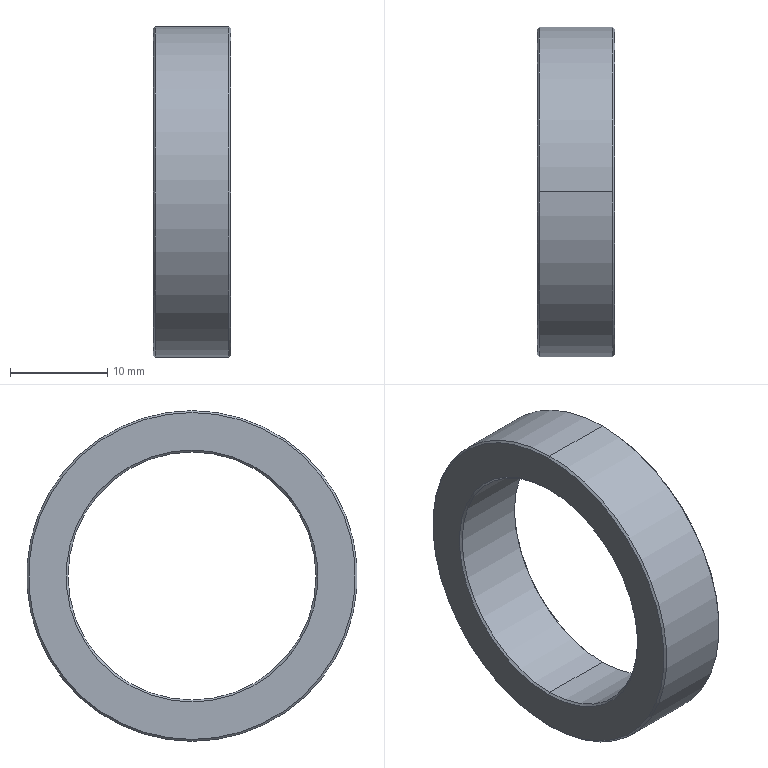Part | SolidWorks | features Chamfer 1, Extrusion 1 | 1 solid | 14 faces | box 8 x 34 x 34 mm | volume 3170 mm3 | cone 8 | cylinder 4 | plane 2 | commonest cylinder face diameters 25.5 x2 34 x2
STEP:
#1=CARTESIAN_POINT('',(-3.8,0.,-12.75));
#2=VERTEX_POINT('',#1);
#3=CARTESIAN_POINT('',(-3.8,0.,12.75));
#4=VERTEX_POINT('',#3);
#5=CARTESIAN_POINT('',(-3.8,0.,0.));
#6=DIRECTION('',(-1.,0.,0.));
#7=DIRECTION('',(0.,0.,-1.));
#8=AXIS2_PLACEMENT_3D('',#5,#6,#7);
#9=CIRCLE('',#8,12.75);
#10=EDGE_CURVE('',#2,#4,#9,.T.);
#11=ORIENTED_EDGE('',*,*,#10,.F.);
#12=CARTESIAN_POINT('',(-4.,0.,-12.95));
#13=VERTEX_POINT('',#12);
#14=CARTESIAN_POINT('',(-4.,0.,-12.95));
#15=DIRECTION('',(-0.7071,0.,-0.7071));
#16=VECTOR('',#15,1000.);
#17=LINE('',#14,#16);
#18=EDGE_CURVE('',#2,#13,#17,.T.);
#19=ORIENTED_EDGE('',*,*,#18,.T.);
#20=CARTESIAN_POINT('',(-4.,0.,12.95));
#21=VERTEX_POINT('',#20);
#22=CARTESIAN_POINT('',(-4.,0.,0.));
#23=DIRECTION('',(1.,0.,0.));
#24=DIRECTION('',(0.,0.,-1.));
#25=AXIS2_PLACEMENT_3D('',#22,#23,#24);
#26=CIRCLE('',#25,12.95);
#27=EDGE_CURVE('',#21,#13,#26,.T.);
#28=ORIENTED_EDGE('',*,*,#27,.F.);
#29=CARTESIAN_POINT('',(-4.,0.,12.95));
#30=DIRECTION('',(-0.7071,0.,0.7071));
#31=VECTOR('',#30,1000.);
#32=LINE('',#29,#31);
#33=EDGE_CURVE('',#4,#21,#32,.T.);
#34=ORIENTED_EDGE('',*,*,#33,.F.);
#35=EDGE_LOOP('',(#11,#19,#28,#34));
#36=FACE_OUTER_BOUND('',#35,.T.);
#37=CARTESIAN_POINT('',(-4.,0.,0.));
#38=DIRECTION('',(-1.,0.,0.));
#39=DIRECTION('',(0.,0.,1.));
#40=AXIS2_PLACEMENT_3D('',#37,#38,#39);
#41=CONICAL_SURFACE('',#40,12.95,0.7854);
#42=ADVANCED_FACE('',(#36),#41,.F.);
#43=CARTESIAN_POINT('',(-4.,0.,16.8));
#44=VERTEX_POINT('',#43);
#45=CARTESIAN_POINT('',(-4.,0.,-16.8));
#46=VERTEX_POINT('',#45);
#47=CARTESIAN_POINT('',(-4.,0.,0.));
#48=DIRECTION('',(-1.,0.,0.));
#49=DIRECTION('',(0.,0.,-1.));
#50=AXIS2_PLACEMENT_3D('',#47,#48,#49);
#51=CIRCLE('',#50,16.8);
#52=EDGE_CURVE('',#44,#46,#51,.T.);
#53=ORIENTED_EDGE('',*,*,#52,.F.);
#54=CARTESIAN_POINT('',(-3.8,0.,17.));
#55=VERTEX_POINT('',#54);
#56=CARTESIAN_POINT('',(-3.8,0.,17.));
#57=DIRECTION('',(0.7071,0.,0.7071));
#58=VECTOR('',#57,1000.);
#59=LINE('',#56,#58);
#60=EDGE_CURVE('',#44,#55,#59,.T.);
#61=ORIENTED_EDGE('',*,*,#60,.T.);
#62=CARTESIAN_POINT('',(-3.8,0.,-17.));
#63=VERTEX_POINT('',#62);
#64=CARTESIAN_POINT('',(-3.8,0.,0.));
#65=DIRECTION('',(1.,0.,0.));
#66=DIRECTION('',(0.,0.,-1.));
#67=AXIS2_PLACEMENT_3D('',#64,#65,#66);
#68=CIRCLE('',#67,17.);
#69=EDGE_CURVE('',#63,#55,#68,.T.);
#70=ORIENTED_EDGE('',*,*,#69,.F.);
#71=CARTESIAN_POINT('',(-3.8,0.,-17.));
#72=DIRECTION('',(0.7071,0.,-0.7071));
#73=VECTOR('',#72,1000.);
#74=LINE('',#71,#73);
#75=EDGE_CURVE('',#46,#63,#74,.T.);
#76=ORIENTED_EDGE('',*,*,#75,.F.);
#77=EDGE_LOOP('',(#53,#61,#70,#76));
#78=FACE_OUTER_BOUND('',#77,.T.);
#79=CARTESIAN_POINT('',(-3.8,0.,0.));
#80=DIRECTION('',(1.,0.,0.));
#81=DIRECTION('',(0.,0.,-1.));
#82=AXIS2_PLACEMENT_3D('',#79,#80,#81);
#83=CONICAL_SURFACE('',#82,17.,0.7854);
#84=ADVANCED_FACE('',(#78),#83,.T.);
#85=CARTESIAN_POINT('',(3.8,0.,12.75));
#86=VERTEX_POINT('',#85);
#87=CARTESIAN_POINT('',(3.8,0.,-12.75));
#88=VERTEX_POINT('',#87);
#89=CARTESIAN_POINT('',(3.8,0.,0.));
#90=DIRECTION('',(1.,0.,0.));
#91=DIRECTION('',(0.,0.,-1.));
#92=AXIS2_PLACEMENT_3D('',#89,#90,#91);
#93=CIRCLE('',#92,12.75);
#94=EDGE_CURVE('',#86,#88,#93,.T.);
#95=ORIENTED_EDGE('',*,*,#94,.F.);
#96=CARTESIAN_POINT('',(4.,0.,12.95));
#97=VERTEX_POINT('',#96);
#98=CARTESIAN_POINT('',(3.8,0.,12.75));
#99=DIRECTION('',(0.7071,0.,0.7071));
#100=VECTOR('',#99,1000.);
#101=LINE('',#98,#100);
#102=EDGE_CURVE('',#86,#97,#101,.T.);
#103=ORIENTED_EDGE('',*,*,#102,.T.);
#104=CARTESIAN_POINT('',(4.,0.,-12.95));
#105=VERTEX_POINT('',#104);
#106=CARTESIAN_POINT('',(4.,0.,0.));
#107=DIRECTION('',(-1.,0.,0.));
#108=DIRECTION('',(0.,0.,-1.));
#109=AXIS2_PLACEMENT_3D('',#106,#107,#108);
#110=CIRCLE('',#109,12.95);
#111=EDGE_CURVE('',#105,#97,#110,.T.);
#112=ORIENTED_EDGE('',*,*,#111,.F.);
#113=CARTESIAN_POINT('',(3.8,0.,-12.75));
#114=DIRECTION('',(0.7071,0.,-0.7071));
#115=VECTOR('',#114,1000.);
#116=LINE('',#113,#115);
#117=EDGE_CURVE('',#88,#105,#116,.T.);
#118=ORIENTED_EDGE('',*,*,#117,.F.);
#119=EDGE_LOOP('',(#95,#103,#112,#118));
#120=FACE_OUTER_BOUND('',#119,.T.);
#121=CARTESIAN_POINT('',(3.8,0.,0.));
#122=DIRECTION('',(1.,0.,0.));
#123=DIRECTION('',(0.,0.,-1.));
#124=AXIS2_PLACEMENT_3D('',#121,#122,#123);
#125=CONICAL_SURFACE('',#124,12.75,0.7854);
#126=ADVANCED_FACE('',(#120),#125,.F.);
#127=CARTESIAN_POINT('',(4.,0.,-16.8));
#128=VERTEX_POINT('',#127);
#129=CARTESIAN_POINT('',(4.,0.,16.8));
#130=VERTEX_POINT('',#129);
#131=CARTESIAN_POINT('',(4.,0.,0.));
#132=DIRECTION('',(1.,0.,0.));
#133=DIRECTION('',(0.,0.,-1.));
#134=AXIS2_PLACEMENT_3D('',#131,#132,#133);
#135=CIRCLE('',#134,16.8);
#136=EDGE_CURVE('',#128,#130,#135,.T.);
#137=ORIENTED_EDGE('',*,*,#136,.F.);
#138=CARTESIAN_POINT('',(3.8,0.,-17.));
#139=VERTEX_POINT('',#138);
#140=CARTESIAN_POINT('',(4.,0.,-16.8));
#141=DIRECTION('',(-0.7071,0.,-0.7071));
#142=VECTOR('',#141,1000.);
#143=LINE('',#140,#142);
#144=EDGE_CURVE('',#128,#139,#143,.T.);
#145=ORIENTED_EDGE('',*,*,#144,.T.);
#146=CARTESIAN_POINT('',(3.8,0.,17.));
#147=VERTEX_POINT('',#146);
#148=CARTESIAN_POINT('',(3.8,0.,0.));
#149=DIRECTION('',(-1.,0.,0.));
#150=DIRECTION('',(0.,0.,-1.));
#151=AXIS2_PLACEMENT_3D('',#148,#149,#150);
#152=CIRCLE('',#151,17.);
#153=EDGE_CURVE('',#147,#139,#152,.T.);
#154=ORIENTED_EDGE('',*,*,#153,.F.);
#155=CARTESIAN_POINT('',(4.,0.,16.8));
#156=DIRECTION('',(-0.7071,0.,0.7071));
#157=VECTOR('',#156,1000.);
#158=LINE('',#155,#157);
#159=EDGE_CURVE('',#130,#147,#158,.T.);
#160=ORIENTED_EDGE('',*,*,#159,.F.);
#161=EDGE_LOOP('',(#137,#145,#154,#160));
#162=FACE_OUTER_BOUND('',#161,.T.);
#163=CARTESIAN_POINT('',(4.,0.,0.));
#164=DIRECTION('',(-1.,0.,0.));
#165=DIRECTION('',(0.,0.,1.));
#166=AXIS2_PLACEMENT_3D('',#163,#164,#165);
#167=CONICAL_SURFACE('',#166,16.8,0.7854);
#168=ADVANCED_FACE('',(#162),#167,.T.);
#169=ORIENTED_EDGE('',*,*,#94,.T.);
#170=CARTESIAN_POINT('',(4.,0.,-12.75));
#171=DIRECTION('',(-1.,0.,0.));
#172=VECTOR('',#171,1000.);
#173=LINE('',#170,#172);
#174=EDGE_CURVE('',#88,#2,#173,.T.);
#175=ORIENTED_EDGE('',*,*,#174,.T.);
#176=ORIENTED_EDGE('',*,*,#10,.T.);
#177=CARTESIAN_POINT('',(4.,0.,12.75));
#178=DIRECTION('',(-1.,0.,0.));
#179=VECTOR('',#178,1000.);
#180=LINE('',#177,#179);
#181=EDGE_CURVE('',#86,#4,#180,.T.);
#182=ORIENTED_EDGE('',*,*,#181,.F.);
#183=EDGE_LOOP('',(#169,#175,#176,#182));
#184=FACE_OUTER_BOUND('',#183,.T.);
#185=CARTESIAN_POINT('',(4.,0.,0.));
#186=DIRECTION('',(-1.,0.,0.));
#187=DIRECTION('',(0.,0.,1.));
#188=AXIS2_PLACEMENT_3D('',#185,#186,#187);
#189=CYLINDRICAL_SURFACE('',#188,12.75);
#190=ADVANCED_FACE('',(#184),#189,.F.);
#191=ORIENTED_EDGE('',*,*,#153,.T.);
#192=CARTESIAN_POINT('',(4.,0.,-17.));
#193=DIRECTION('',(-1.,0.,0.));
#194=VECTOR('',#193,1000.);
#195=LINE('',#192,#194);
#196=EDGE_CURVE('',#139,#63,#195,.T.);
#197=ORIENTED_EDGE('',*,*,#196,.T.);
#198=ORIENTED_EDGE('',*,*,#69,.T.);
#199=CARTESIAN_POINT('',(4.,0.,17.));
#200=DIRECTION('',(-1.,0.,0.));
#201=VECTOR('',#200,1000.);
#202=LINE('',#199,#201);
#203=EDGE_CURVE('',#147,#55,#202,.T.);
#204=ORIENTED_EDGE('',*,*,#203,.F.);
#205=EDGE_LOOP('',(#191,#197,#198,#204));
#206=FACE_OUTER_BOUND('',#205,.T.);
#207=CARTESIAN_POINT('',(4.,0.,0.));
#208=DIRECTION('',(-1.,0.,0.));
#209=DIRECTION('',(0.,0.,1.));
#210=AXIS2_PLACEMENT_3D('',#207,#208,#209);
#211=CYLINDRICAL_SURFACE('',#210,17.);
#212=ADVANCED_FACE('',(#206),#211,.T.);
#213=CARTESIAN_POINT('',(4.,0.,0.));
#214=DIRECTION('',(1.,0.,0.));
#215=DIRECTION('',(0.,0.,-1.));
#216=AXIS2_PLACEMENT_3D('',#213,#214,#215);
#217=CIRCLE('',#216,16.8);
#218=EDGE_CURVE('',#130,#128,#217,.T.);
#219=ORIENTED_EDGE('',*,*,#218,.T.);
#220=ORIENTED_EDGE('',*,*,#136,.T.);
#221=EDGE_LOOP('',(#219,#220));
#222=FACE_OUTER_BOUND('',#221,.T.);
#223=ORIENTED_EDGE('',*,*,#111,.T.);
#224=CARTESIAN_POINT('',(4.,0.,0.));
#225=DIRECTION('',(-1.,0.,0.));
#226=DIRECTION('',(0.,0.,-1.));
#227=AXIS2_PLACEMENT_3D('',#224,#225,#226);
#228=CIRCLE('',#227,12.95);
#229=EDGE_CURVE('',#97,#105,#228,.T.);
#230=ORIENTED_EDGE('',*,*,#229,.T.);
#231=EDGE_LOOP('',(#223,#230));
#232=FACE_BOUND('',#231,.T.);
#233=CARTESIAN_POINT('',(4.,0.,0.));
#234=DIRECTION('',(1.,0.,0.));
#235=DIRECTION('',(0.,0.,-1.));
#236=AXIS2_PLACEMENT_3D('',#233,#234,#235);
#237=PLANE('',#236);
#238=ADVANCED_FACE('',(#222,#232),#237,.T.);
#239=CARTESIAN_POINT('',(-4.,0.,0.));
#240=DIRECTION('',(-1.,0.,0.));
#241=DIRECTION('',(0.,0.,-1.));
#242=AXIS2_PLACEMENT_3D('',#239,#240,#241);
#243=CIRCLE('',#242,16.8);
#244=EDGE_CURVE('',#46,#44,#243,.T.);
#245=ORIENTED_EDGE('',*,*,#244,.T.);
#246=ORIENTED_EDGE('',*,*,#52,.T.);
#247=EDGE_LOOP('',(#245,#246));
#248=FACE_OUTER_BOUND('',#247,.T.);
#249=ORIENTED_EDGE('',*,*,#27,.T.);
#250=CARTESIAN_POINT('',(-4.,0.,0.));
#251=DIRECTION('',(1.,0.,0.));
#252=DIRECTION('',(0.,0.,-1.));
#253=AXIS2_PLACEMENT_3D('',#250,#251,#252);
#254=CIRCLE('',#253,12.95);
#255=EDGE_CURVE('',#13,#21,#254,.T.);
#256=ORIENTED_EDGE('',*,*,#255,.T.);
#257=EDGE_LOOP('',(#249,#256));
#258=FACE_BOUND('',#257,.T.);
#259=CARTESIAN_POINT('',(-4.,0.,0.));
#260=DIRECTION('',(1.,0.,0.));
#261=DIRECTION('',(0.,0.,-1.));
#262=AXIS2_PLACEMENT_3D('',#259,#260,#261);
#263=PLANE('',#262);
#264=ADVANCED_FACE('',(#248,#258),#263,.F.);
#265=ORIENTED_EDGE('',*,*,#196,.F.);
#266=CARTESIAN_POINT('',(3.8,0.,0.));
#267=DIRECTION('',(-1.,0.,0.));
#268=DIRECTION('',(0.,0.,-1.));
#269=AXIS2_PLACEMENT_3D('',#266,#267,#268);
#270=CIRCLE('',#269,17.);
#271=EDGE_CURVE('',#139,#147,#270,.T.);
#272=ORIENTED_EDGE('',*,*,#271,.T.);
#273=ORIENTED_EDGE('',*,*,#203,.T.);
#274=CARTESIAN_POINT('',(-3.8,0.,0.));
#275=DIRECTION('',(1.,0.,0.));
#276=DIRECTION('',(0.,0.,-1.));
#277=AXIS2_PLACEMENT_3D('',#274,#275,#276);
#278=CIRCLE('',#277,17.);
#279=EDGE_CURVE('',#55,#63,#278,.T.);
#280=ORIENTED_EDGE('',*,*,#279,.T.);
#281=EDGE_LOOP('',(#265,#272,#273,#280));
#282=FACE_OUTER_BOUND('',#281,.T.);
#283=CARTESIAN_POINT('',(4.,0.,0.));
#284=DIRECTION('',(-1.,0.,0.));
#285=DIRECTION('',(0.,0.,1.));
#286=AXIS2_PLACEMENT_3D('',#283,#284,#285);
#287=CYLINDRICAL_SURFACE('',#286,17.);
#288=ADVANCED_FACE('',(#282),#287,.T.);
#289=ORIENTED_EDGE('',*,*,#174,.F.);
#290=CARTESIAN_POINT('',(3.8,0.,0.));
#291=DIRECTION('',(1.,0.,0.));
#292=DIRECTION('',(0.,0.,-1.));
#293=AXIS2_PLACEMENT_3D('',#290,#291,#292);
#294=CIRCLE('',#293,12.75);
#295=EDGE_CURVE('',#88,#86,#294,.T.);
#296=ORIENTED_EDGE('',*,*,#295,.T.);
#297=ORIENTED_EDGE('',*,*,#181,.T.);
#298=CARTESIAN_POINT('',(-3.8,0.,0.));
#299=DIRECTION('',(-1.,0.,0.));
#300=DIRECTION('',(0.,0.,-1.));
#301=AXIS2_PLACEMENT_3D('',#298,#299,#300);
#302=CIRCLE('',#301,12.75);
#303=EDGE_CURVE('',#4,#2,#302,.T.);
#304=ORIENTED_EDGE('',*,*,#303,.T.);
#305=EDGE_LOOP('',(#289,#296,#297,#304));
#306=FACE_OUTER_BOUND('',#305,.T.);
#307=CARTESIAN_POINT('',(4.,0.,0.));
#308=DIRECTION('',(-1.,0.,0.));
#309=DIRECTION('',(0.,0.,1.));
#310=AXIS2_PLACEMENT_3D('',#307,#308,#309);
#311=CYLINDRICAL_SURFACE('',#310,12.75);
#312=ADVANCED_FACE('',(#306),#311,.F.);
#313=ORIENTED_EDGE('',*,*,#144,.F.);
#314=ORIENTED_EDGE('',*,*,#218,.F.);
#315=ORIENTED_EDGE('',*,*,#159,.T.);
#316=ORIENTED_EDGE('',*,*,#271,.F.);
#317=EDGE_LOOP('',(#313,#314,#315,#316));
#318=FACE_OUTER_BOUND('',#317,.T.);
#319=CARTESIAN_POINT('',(4.,0.,0.));
#320=DIRECTION('',(-1.,0.,0.));
#321=DIRECTION('',(0.,0.,1.));
#322=AXIS2_PLACEMENT_3D('',#319,#320,#321);
#323=CONICAL_SURFACE('',#322,16.8,0.7854);
#324=ADVANCED_FACE('',(#318),#323,.T.);
#325=ORIENTED_EDGE('',*,*,#102,.F.);
#326=ORIENTED_EDGE('',*,*,#295,.F.);
#327=ORIENTED_EDGE('',*,*,#117,.T.);
#328=ORIENTED_EDGE('',*,*,#229,.F.);
#329=EDGE_LOOP('',(#325,#326,#327,#328));
#330=FACE_OUTER_BOUND('',#329,.T.);
#331=CARTESIAN_POINT('',(3.8,0.,0.));
#332=DIRECTION('',(1.,0.,0.));
#333=DIRECTION('',(0.,0.,-1.));
#334=AXIS2_PLACEMENT_3D('',#331,#332,#333);
#335=CONICAL_SURFACE('',#334,12.75,0.7854);
#336=ADVANCED_FACE('',(#330),#335,.F.);
#337=ORIENTED_EDGE('',*,*,#60,.F.);
#338=ORIENTED_EDGE('',*,*,#244,.F.);
#339=ORIENTED_EDGE('',*,*,#75,.T.);
#340=ORIENTED_EDGE('',*,*,#279,.F.);
#341=EDGE_LOOP('',(#337,#338,#339,#340));
#342=FACE_OUTER_BOUND('',#341,.T.);
#343=CARTESIAN_POINT('',(-3.8,0.,0.));
#344=DIRECTION('',(1.,0.,0.));
#345=DIRECTION('',(0.,0.,-1.));
#346=AXIS2_PLACEMENT_3D('',#343,#344,#345);
#347=CONICAL_SURFACE('',#346,17.,0.7854);
#348=ADVANCED_FACE('',(#342),#347,.T.);
#349=ORIENTED_EDGE('',*,*,#18,.F.);
#350=ORIENTED_EDGE('',*,*,#303,.F.);
#351=ORIENTED_EDGE('',*,*,#33,.T.);
#352=ORIENTED_EDGE('',*,*,#255,.F.);
#353=EDGE_LOOP('',(#349,#350,#351,#352));
#354=FACE_OUTER_BOUND('',#353,.T.);
#355=CARTESIAN_POINT('',(-4.,0.,0.));
#356=DIRECTION('',(-1.,0.,0.));
#357=DIRECTION('',(0.,0.,1.));
#358=AXIS2_PLACEMENT_3D('',#355,#356,#357);
#359=CONICAL_SURFACE('',#358,12.95,0.7854);
#360=ADVANCED_FACE('',(#354),#359,.F.);
#361=CLOSED_SHELL('',(#42,#84,#126,#168,#190,#212,#238,#264,#288,#312,#324,#336,#348,#360));
#362=MANIFOLD_SOLID_BREP('',#361);
#363=CARTESIAN_POINT('',(0.,0.,0.));
#364=DIRECTION('',(0.,0.,1.));
#365=DIRECTION('',(1.,0.,0.));
#366=AXIS2_PLACEMENT_3D('',#363,#364,#365);
#367=(LENGTH_UNIT()NAMED_UNIT(*)SI_UNIT(.MILLI.,.METRE.));
#368=UNCERTAINTY_MEASURE_WITH_UNIT(LENGTH_MEASURE(0.00001),#367,'','');
#369=(NAMED_UNIT(*)PLANE_ANGLE_UNIT()SI_UNIT($,.RADIAN.));
#370=(NAMED_UNIT(*)SI_UNIT($,.STERADIAN.)SOLID_ANGLE_UNIT());
#371=(GEOMETRIC_REPRESENTATION_CONTEXT(3)GLOBAL_UNCERTAINTY_ASSIGNED_CONTEXT((#368))GLOBAL_UNIT_ASSIGNED_CONTEXT((#367,#369,#370))REPRESENTATION_CONTEXT('',''));
#372=ADVANCED_BREP_SHAPE_REPRESENTATION('',(#362,#366),#371);